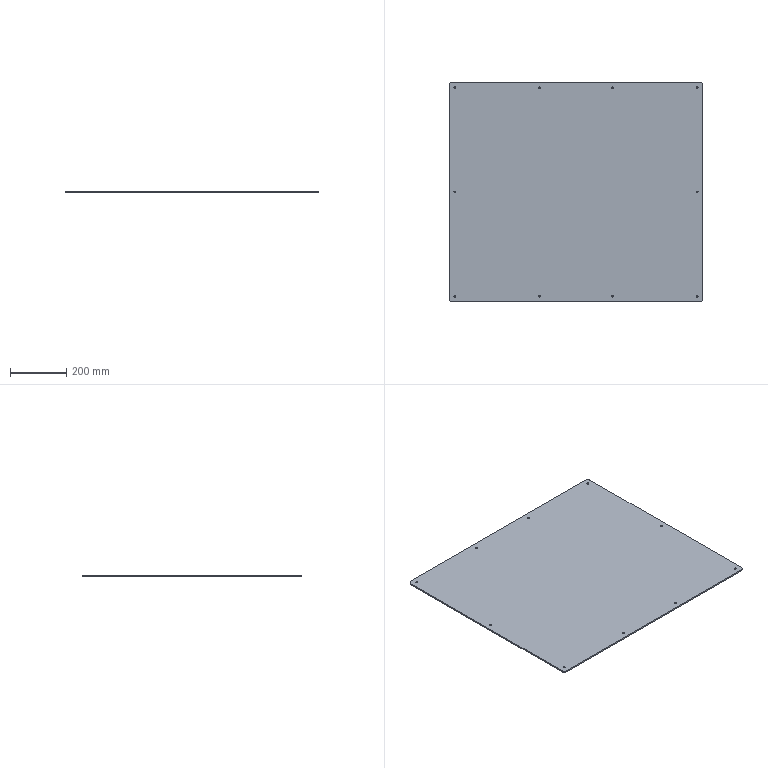Part | SolidWorks | features Extrusion 1, Fillet 1, HoleWzd 1 | 1 solid | 30 faces | box 900 x 780 x 5 mm | volume 3507647 mm3 | cylinder 24 | plane 6 | commonest cylinder face diameters 7 x20 20 x4
STEP:
#1=CARTESIAN_POINT('',(-426.5,370.,0.));
#2=VERTEX_POINT('',#1);
#3=CARTESIAN_POINT('',(-433.5,370.,0.));
#4=VERTEX_POINT('',#3);
#5=CARTESIAN_POINT('',(-430.,370.,0.));
#6=DIRECTION('',(0.,0.,-1.));
#7=DIRECTION('',(-1.,0.,0.));
#8=AXIS2_PLACEMENT_3D('',#5,#6,#7);
#9=CIRCLE('',#8,3.5);
#10=EDGE_CURVE('',#2,#4,#9,.T.);
#11=ORIENTED_EDGE('',*,*,#10,.T.);
#12=CARTESIAN_POINT('',(-433.5,370.,5.));
#13=VERTEX_POINT('',#12);
#14=CARTESIAN_POINT('',(-433.5,370.,5.));
#15=DIRECTION('',(0.,0.,1.));
#16=VECTOR('',#15,1000.);
#17=LINE('',#14,#16);
#18=EDGE_CURVE('',#4,#13,#17,.T.);
#19=ORIENTED_EDGE('',*,*,#18,.T.);
#20=CARTESIAN_POINT('',(-426.5,370.,5.));
#21=VERTEX_POINT('',#20);
#22=CARTESIAN_POINT('',(-430.,370.,5.));
#23=DIRECTION('',(0.,0.,1.));
#24=DIRECTION('',(1.,0.,0.));
#25=AXIS2_PLACEMENT_3D('',#22,#23,#24);
#26=CIRCLE('',#25,3.5);
#27=EDGE_CURVE('',#13,#21,#26,.T.);
#28=ORIENTED_EDGE('',*,*,#27,.T.);
#29=CARTESIAN_POINT('',(-426.5,370.,5.));
#30=DIRECTION('',(0.,0.,1.));
#31=VECTOR('',#30,1000.);
#32=LINE('',#29,#31);
#33=EDGE_CURVE('',#2,#21,#32,.T.);
#34=ORIENTED_EDGE('',*,*,#33,.F.);
#35=EDGE_LOOP('',(#11,#19,#28,#34));
#36=FACE_OUTER_BOUND('',#35,.T.);
#37=CARTESIAN_POINT('',(-430.,370.,5.));
#38=DIRECTION('',(0.,0.,1.));
#39=DIRECTION('',(1.,0.,0.));
#40=AXIS2_PLACEMENT_3D('',#37,#38,#39);
#41=CYLINDRICAL_SURFACE('',#40,3.5);
#42=ADVANCED_FACE('',(#36),#41,.F.);
#43=CARTESIAN_POINT('',(433.5,370.,0.));
#44=VERTEX_POINT('',#43);
#45=CARTESIAN_POINT('',(426.5,370.,0.));
#46=VERTEX_POINT('',#45);
#47=CARTESIAN_POINT('',(430.,370.,0.));
#48=DIRECTION('',(0.,0.,-1.));
#49=DIRECTION('',(-1.,0.,0.));
#50=AXIS2_PLACEMENT_3D('',#47,#48,#49);
#51=CIRCLE('',#50,3.5);
#52=EDGE_CURVE('',#44,#46,#51,.T.);
#53=ORIENTED_EDGE('',*,*,#52,.T.);
#54=CARTESIAN_POINT('',(426.5,370.,5.));
#55=VERTEX_POINT('',#54);
#56=CARTESIAN_POINT('',(426.5,370.,5.));
#57=DIRECTION('',(0.,0.,1.));
#58=VECTOR('',#57,1000.);
#59=LINE('',#56,#58);
#60=EDGE_CURVE('',#46,#55,#59,.T.);
#61=ORIENTED_EDGE('',*,*,#60,.T.);
#62=CARTESIAN_POINT('',(433.5,370.,5.));
#63=VERTEX_POINT('',#62);
#64=CARTESIAN_POINT('',(430.,370.,5.));
#65=DIRECTION('',(0.,0.,1.));
#66=DIRECTION('',(1.,0.,0.));
#67=AXIS2_PLACEMENT_3D('',#64,#65,#66);
#68=CIRCLE('',#67,3.5);
#69=EDGE_CURVE('',#55,#63,#68,.T.);
#70=ORIENTED_EDGE('',*,*,#69,.T.);
#71=CARTESIAN_POINT('',(433.5,370.,5.));
#72=DIRECTION('',(0.,0.,1.));
#73=VECTOR('',#72,1000.);
#74=LINE('',#71,#73);
#75=EDGE_CURVE('',#44,#63,#74,.T.);
#76=ORIENTED_EDGE('',*,*,#75,.F.);
#77=EDGE_LOOP('',(#53,#61,#70,#76));
#78=FACE_OUTER_BOUND('',#77,.T.);
#79=CARTESIAN_POINT('',(430.,370.,5.));
#80=DIRECTION('',(0.,0.,1.));
#81=DIRECTION('',(1.,0.,0.));
#82=AXIS2_PLACEMENT_3D('',#79,#80,#81);
#83=CYLINDRICAL_SURFACE('',#82,3.5);
#84=ADVANCED_FACE('',(#78),#83,.F.);
#85=CARTESIAN_POINT('',(433.5,-370.,0.));
#86=VERTEX_POINT('',#85);
#87=CARTESIAN_POINT('',(426.5,-370.,0.));
#88=VERTEX_POINT('',#87);
#89=CARTESIAN_POINT('',(430.,-370.,0.));
#90=DIRECTION('',(0.,0.,-1.));
#91=DIRECTION('',(-1.,0.,0.));
#92=AXIS2_PLACEMENT_3D('',#89,#90,#91);
#93=CIRCLE('',#92,3.5);
#94=EDGE_CURVE('',#86,#88,#93,.T.);
#95=ORIENTED_EDGE('',*,*,#94,.T.);
#96=CARTESIAN_POINT('',(426.5,-370.,5.));
#97=VERTEX_POINT('',#96);
#98=CARTESIAN_POINT('',(426.5,-370.,5.));
#99=DIRECTION('',(0.,0.,1.));
#100=VECTOR('',#99,1000.);
#101=LINE('',#98,#100);
#102=EDGE_CURVE('',#88,#97,#101,.T.);
#103=ORIENTED_EDGE('',*,*,#102,.T.);
#104=CARTESIAN_POINT('',(433.5,-370.,5.));
#105=VERTEX_POINT('',#104);
#106=CARTESIAN_POINT('',(430.,-370.,5.));
#107=DIRECTION('',(0.,0.,1.));
#108=DIRECTION('',(1.,0.,0.));
#109=AXIS2_PLACEMENT_3D('',#106,#107,#108);
#110=CIRCLE('',#109,3.5);
#111=EDGE_CURVE('',#97,#105,#110,.T.);
#112=ORIENTED_EDGE('',*,*,#111,.T.);
#113=CARTESIAN_POINT('',(433.5,-370.,5.));
#114=DIRECTION('',(0.,0.,1.));
#115=VECTOR('',#114,1000.);
#116=LINE('',#113,#115);
#117=EDGE_CURVE('',#86,#105,#116,.T.);
#118=ORIENTED_EDGE('',*,*,#117,.F.);
#119=EDGE_LOOP('',(#95,#103,#112,#118));
#120=FACE_OUTER_BOUND('',#119,.T.);
#121=CARTESIAN_POINT('',(430.,-370.,5.));
#122=DIRECTION('',(0.,0.,1.));
#123=DIRECTION('',(1.,0.,0.));
#124=AXIS2_PLACEMENT_3D('',#121,#122,#123);
#125=CYLINDRICAL_SURFACE('',#124,3.5);
#126=ADVANCED_FACE('',(#120),#125,.F.);
#127=CARTESIAN_POINT('',(-426.5,-370.,0.));
#128=VERTEX_POINT('',#127);
#129=CARTESIAN_POINT('',(-433.5,-370.,0.));
#130=VERTEX_POINT('',#129);
#131=CARTESIAN_POINT('',(-430.,-370.,0.));
#132=DIRECTION('',(0.,0.,-1.));
#133=DIRECTION('',(-1.,0.,0.));
#134=AXIS2_PLACEMENT_3D('',#131,#132,#133);
#135=CIRCLE('',#134,3.5);
#136=EDGE_CURVE('',#128,#130,#135,.T.);
#137=ORIENTED_EDGE('',*,*,#136,.T.);
#138=CARTESIAN_POINT('',(-433.5,-370.,5.));
#139=VERTEX_POINT('',#138);
#140=CARTESIAN_POINT('',(-433.5,-370.,5.));
#141=DIRECTION('',(0.,0.,1.));
#142=VECTOR('',#141,1000.);
#143=LINE('',#140,#142);
#144=EDGE_CURVE('',#130,#139,#143,.T.);
#145=ORIENTED_EDGE('',*,*,#144,.T.);
#146=CARTESIAN_POINT('',(-426.5,-370.,5.));
#147=VERTEX_POINT('',#146);
#148=CARTESIAN_POINT('',(-430.,-370.,5.));
#149=DIRECTION('',(0.,0.,1.));
#150=DIRECTION('',(1.,0.,0.));
#151=AXIS2_PLACEMENT_3D('',#148,#149,#150);
#152=CIRCLE('',#151,3.5);
#153=EDGE_CURVE('',#139,#147,#152,.T.);
#154=ORIENTED_EDGE('',*,*,#153,.T.);
#155=CARTESIAN_POINT('',(-426.5,-370.,5.));
#156=DIRECTION('',(0.,0.,1.));
#157=VECTOR('',#156,1000.);
#158=LINE('',#155,#157);
#159=EDGE_CURVE('',#128,#147,#158,.T.);
#160=ORIENTED_EDGE('',*,*,#159,.F.);
#161=EDGE_LOOP('',(#137,#145,#154,#160));
#162=FACE_OUTER_BOUND('',#161,.T.);
#163=CARTESIAN_POINT('',(-430.,-370.,5.));
#164=DIRECTION('',(0.,0.,1.));
#165=DIRECTION('',(1.,0.,0.));
#166=AXIS2_PLACEMENT_3D('',#163,#164,#165);
#167=CYLINDRICAL_SURFACE('',#166,3.5);
#168=ADVANCED_FACE('',(#162),#167,.F.);
#169=CARTESIAN_POINT('',(-426.5,0.,0.));
#170=VERTEX_POINT('',#169);
#171=CARTESIAN_POINT('',(-433.5,0.,0.));
#172=VERTEX_POINT('',#171);
#173=CARTESIAN_POINT('',(-430.,0.,0.));
#174=DIRECTION('',(0.,0.,-1.));
#175=DIRECTION('',(-1.,0.,0.));
#176=AXIS2_PLACEMENT_3D('',#173,#174,#175);
#177=CIRCLE('',#176,3.5);
#178=EDGE_CURVE('',#170,#172,#177,.T.);
#179=ORIENTED_EDGE('',*,*,#178,.T.);
#180=CARTESIAN_POINT('',(-433.5,0.,5.));
#181=VERTEX_POINT('',#180);
#182=CARTESIAN_POINT('',(-433.5,0.,5.));
#183=DIRECTION('',(0.,0.,1.));
#184=VECTOR('',#183,1000.);
#185=LINE('',#182,#184);
#186=EDGE_CURVE('',#172,#181,#185,.T.);
#187=ORIENTED_EDGE('',*,*,#186,.T.);
#188=CARTESIAN_POINT('',(-426.5,0.,5.));
#189=VERTEX_POINT('',#188);
#190=CARTESIAN_POINT('',(-430.,0.,5.));
#191=DIRECTION('',(0.,0.,1.));
#192=DIRECTION('',(1.,0.,0.));
#193=AXIS2_PLACEMENT_3D('',#190,#191,#192);
#194=CIRCLE('',#193,3.5);
#195=EDGE_CURVE('',#181,#189,#194,.T.);
#196=ORIENTED_EDGE('',*,*,#195,.T.);
#197=CARTESIAN_POINT('',(-426.5,0.,5.));
#198=DIRECTION('',(0.,0.,1.));
#199=VECTOR('',#198,1000.);
#200=LINE('',#197,#199);
#201=EDGE_CURVE('',#170,#189,#200,.T.);
#202=ORIENTED_EDGE('',*,*,#201,.F.);
#203=EDGE_LOOP('',(#179,#187,#196,#202));
#204=FACE_OUTER_BOUND('',#203,.T.);
#205=CARTESIAN_POINT('',(-430.,0.,5.));
#206=DIRECTION('',(0.,0.,1.));
#207=DIRECTION('',(1.,0.,0.));
#208=AXIS2_PLACEMENT_3D('',#205,#206,#207);
#209=CYLINDRICAL_SURFACE('',#208,3.5);
#210=ADVANCED_FACE('',(#204),#209,.F.);
#211=CARTESIAN_POINT('',(433.5,0.,0.));
#212=VERTEX_POINT('',#211);
#213=CARTESIAN_POINT('',(426.5,0.,0.));
#214=VERTEX_POINT('',#213);
#215=CARTESIAN_POINT('',(430.,0.,0.));
#216=DIRECTION('',(0.,0.,-1.));
#217=DIRECTION('',(-1.,0.,0.));
#218=AXIS2_PLACEMENT_3D('',#215,#216,#217);
#219=CIRCLE('',#218,3.5);
#220=EDGE_CURVE('',#212,#214,#219,.T.);
#221=ORIENTED_EDGE('',*,*,#220,.T.);
#222=CARTESIAN_POINT('',(426.5,0.,5.));
#223=VERTEX_POINT('',#222);
#224=CARTESIAN_POINT('',(426.5,0.,5.));
#225=DIRECTION('',(0.,0.,1.));
#226=VECTOR('',#225,1000.);
#227=LINE('',#224,#226);
#228=EDGE_CURVE('',#214,#223,#227,.T.);
#229=ORIENTED_EDGE('',*,*,#228,.T.);
#230=CARTESIAN_POINT('',(433.5,0.,5.));
#231=VERTEX_POINT('',#230);
#232=CARTESIAN_POINT('',(430.,0.,5.));
#233=DIRECTION('',(0.,0.,1.));
#234=DIRECTION('',(1.,0.,0.));
#235=AXIS2_PLACEMENT_3D('',#232,#233,#234);
#236=CIRCLE('',#235,3.5);
#237=EDGE_CURVE('',#223,#231,#236,.T.);
#238=ORIENTED_EDGE('',*,*,#237,.T.);
#239=CARTESIAN_POINT('',(433.5,0.,5.));
#240=DIRECTION('',(0.,0.,1.));
#241=VECTOR('',#240,1000.);
#242=LINE('',#239,#241);
#243=EDGE_CURVE('',#212,#231,#242,.T.);
#244=ORIENTED_EDGE('',*,*,#243,.F.);
#245=EDGE_LOOP('',(#221,#229,#238,#244));
#246=FACE_OUTER_BOUND('',#245,.T.);
#247=CARTESIAN_POINT('',(430.,0.,5.));
#248=DIRECTION('',(0.,0.,1.));
#249=DIRECTION('',(1.,0.,0.));
#250=AXIS2_PLACEMENT_3D('',#247,#248,#249);
#251=CYLINDRICAL_SURFACE('',#250,3.5);
#252=ADVANCED_FACE('',(#246),#251,.F.);
#253=CARTESIAN_POINT('',(-126.5,370.,0.));
#254=VERTEX_POINT('',#253);
#255=CARTESIAN_POINT('',(-133.5,370.,0.));
#256=VERTEX_POINT('',#255);
#257=CARTESIAN_POINT('',(-130.,370.,0.));
#258=DIRECTION('',(0.,0.,-1.));
#259=DIRECTION('',(-1.,0.,0.));
#260=AXIS2_PLACEMENT_3D('',#257,#258,#259);
#261=CIRCLE('',#260,3.5);
#262=EDGE_CURVE('',#254,#256,#261,.T.);
#263=ORIENTED_EDGE('',*,*,#262,.T.);
#264=CARTESIAN_POINT('',(-133.5,370.,5.));
#265=VERTEX_POINT('',#264);
#266=CARTESIAN_POINT('',(-133.5,370.,5.));
#267=DIRECTION('',(0.,0.,1.));
#268=VECTOR('',#267,1000.);
#269=LINE('',#266,#268);
#270=EDGE_CURVE('',#256,#265,#269,.T.);
#271=ORIENTED_EDGE('',*,*,#270,.T.);
#272=CARTESIAN_POINT('',(-126.5,370.,5.));
#273=VERTEX_POINT('',#272);
#274=CARTESIAN_POINT('',(-130.,370.,5.));
#275=DIRECTION('',(0.,0.,1.));
#276=DIRECTION('',(1.,0.,0.));
#277=AXIS2_PLACEMENT_3D('',#274,#275,#276);
#278=CIRCLE('',#277,3.5);
#279=EDGE_CURVE('',#265,#273,#278,.T.);
#280=ORIENTED_EDGE('',*,*,#279,.T.);
#281=CARTESIAN_POINT('',(-126.5,370.,5.));
#282=DIRECTION('',(0.,0.,1.));
#283=VECTOR('',#282,1000.);
#284=LINE('',#281,#283);
#285=EDGE_CURVE('',#254,#273,#284,.T.);
#286=ORIENTED_EDGE('',*,*,#285,.F.);
#287=EDGE_LOOP('',(#263,#271,#280,#286));
#288=FACE_OUTER_BOUND('',#287,.T.);
#289=CARTESIAN_POINT('',(-130.,370.,5.));
#290=DIRECTION('',(0.,0.,1.));
#291=DIRECTION('',(1.,0.,0.));
#292=AXIS2_PLACEMENT_3D('',#289,#290,#291);
#293=CYLINDRICAL_SURFACE('',#292,3.5);
#294=ADVANCED_FACE('',(#288),#293,.F.);
#295=CARTESIAN_POINT('',(133.5,370.,0.));
#296=VERTEX_POINT('',#295);
#297=CARTESIAN_POINT('',(126.5,370.,0.));
#298=VERTEX_POINT('',#297);
#299=CARTESIAN_POINT('',(130.,370.,0.));
#300=DIRECTION('',(0.,0.,-1.));
#301=DIRECTION('',(-1.,0.,0.));
#302=AXIS2_PLACEMENT_3D('',#299,#300,#301);
#303=CIRCLE('',#302,3.5);
#304=EDGE_CURVE('',#296,#298,#303,.T.);
#305=ORIENTED_EDGE('',*,*,#304,.T.);
#306=CARTESIAN_POINT('',(126.5,370.,5.));
#307=VERTEX_POINT('',#306);
#308=CARTESIAN_POINT('',(126.5,370.,5.));
#309=DIRECTION('',(0.,0.,1.));
#310=VECTOR('',#309,1000.);
#311=LINE('',#308,#310);
#312=EDGE_CURVE('',#298,#307,#311,.T.);
#313=ORIENTED_EDGE('',*,*,#312,.T.);
#314=CARTESIAN_POINT('',(133.5,370.,5.));
#315=VERTEX_POINT('',#314);
#316=CARTESIAN_POINT('',(130.,370.,5.));
#317=DIRECTION('',(0.,0.,1.));
#318=DIRECTION('',(1.,0.,0.));
#319=AXIS2_PLACEMENT_3D('',#316,#317,#318);
#320=CIRCLE('',#319,3.5);
#321=EDGE_CURVE('',#307,#315,#320,.T.);
#322=ORIENTED_EDGE('',*,*,#321,.T.);
#323=CARTESIAN_POINT('',(133.5,370.,5.));
#324=DIRECTION('',(0.,0.,1.));
#325=VECTOR('',#324,1000.);
#326=LINE('',#323,#325);
#327=EDGE_CURVE('',#296,#315,#326,.T.);
#328=ORIENTED_EDGE('',*,*,#327,.F.);
#329=EDGE_LOOP('',(#305,#313,#322,#328));
#330=FACE_OUTER_BOUND('',#329,.T.);
#331=CARTESIAN_POINT('',(130.,370.,5.));
#332=DIRECTION('',(0.,0.,1.));
#333=DIRECTION('',(1.,0.,0.));
#334=AXIS2_PLACEMENT_3D('',#331,#332,#333);
#335=CYLINDRICAL_SURFACE('',#334,3.5);
#336=ADVANCED_FACE('',(#330),#335,.F.);
#337=CARTESIAN_POINT('',(-126.5,-370.,0.));
#338=VERTEX_POINT('',#337);
#339=CARTESIAN_POINT('',(-133.5,-370.,0.));
#340=VERTEX_POINT('',#339);
#341=CARTESIAN_POINT('',(-130.,-370.,0.));
#342=DIRECTION('',(0.,0.,-1.));
#343=DIRECTION('',(-1.,0.,0.));
#344=AXIS2_PLACEMENT_3D('',#341,#342,#343);
#345=CIRCLE('',#344,3.5);
#346=EDGE_CURVE('',#338,#340,#345,.T.);
#347=ORIENTED_EDGE('',*,*,#346,.T.);
#348=CARTESIAN_POINT('',(-133.5,-370.,5.));
#349=VERTEX_POINT('',#348);
#350=CARTESIAN_POINT('',(-133.5,-370.,5.));
#351=DIRECTION('',(0.,0.,1.));
#352=VECTOR('',#351,1000.);
#353=LINE('',#350,#352);
#354=EDGE_CURVE('',#340,#349,#353,.T.);
#355=ORIENTED_EDGE('',*,*,#354,.T.);
#356=CARTESIAN_POINT('',(-126.5,-370.,5.));
#357=VERTEX_POINT('',#356);
#358=CARTESIAN_POINT('',(-130.,-370.,5.));
#359=DIRECTION('',(0.,0.,1.));
#360=DIRECTION('',(1.,0.,0.));
#361=AXIS2_PLACEMENT_3D('',#358,#359,#360);
#362=CIRCLE('',#361,3.5);
#363=EDGE_CURVE('',#349,#357,#362,.T.);
#364=ORIENTED_EDGE('',*,*,#363,.T.);
#365=CARTESIAN_POINT('',(-126.5,-370.,5.));
#366=DIRECTION('',(0.,0.,1.));
#367=VECTOR('',#366,1000.);
#368=LINE('',#365,#367);
#369=EDGE_CURVE('',#338,#357,#368,.T.);
#370=ORIENTED_EDGE('',*,*,#369,.F.);
#371=EDGE_LOOP('',(#347,#355,#364,#370));
#372=FACE_OUTER_BOUND('',#371,.T.);
#373=CARTESIAN_POINT('',(-130.,-370.,5.));
#374=DIRECTION('',(0.,0.,1.));
#375=DIRECTION('',(1.,0.,0.));
#376=AXIS2_PLACEMENT_3D('',#373,#374,#375);
#377=CYLINDRICAL_SURFACE('',#376,3.5);
#378=ADVANCED_FACE('',(#372),#377,.F.);
#379=CARTESIAN_POINT('',(133.5,-370.,0.));
#380=VERTEX_POINT('',#379);
#381=CARTESIAN_POINT('',(126.5,-370.,0.));
#382=VERTEX_POINT('',#381);
#383=CARTESIAN_POINT('',(130.,-370.,0.));
#384=DIRECTION('',(0.,0.,-1.));
#385=DIRECTION('',(-1.,0.,0.));
#386=AXIS2_PLACEMENT_3D('',#383,#384,#385);
#387=CIRCLE('',#386,3.5);
#388=EDGE_CURVE('',#380,#382,#387,.T.);
#389=ORIENTED_EDGE('',*,*,#388,.T.);
#390=CARTESIAN_POINT('',(126.5,-370.,5.));
#391=VERTEX_POINT('',#390);
#392=CARTESIAN_POINT('',(126.5,-370.,5.));
#393=DIRECTION('',(0.,0.,1.));
#394=VECTOR('',#393,1000.);
#395=LINE('',#392,#394);
#396=EDGE_CURVE('',#382,#391,#395,.T.);
#397=ORIENTED_EDGE('',*,*,#396,.T.);
#398=CARTESIAN_POINT('',(133.5,-370.,5.));
#399=VERTEX_POINT('',#398);
#400=CARTESIAN_POINT('',(130.,-370.,5.));
#401=DIRECTION('',(0.,0.,1.));
#402=DIRECTION('',(1.,0.,0.));
#403=AXIS2_PLACEMENT_3D('',#400,#401,#402);
#404=CIRCLE('',#403,3.5);
#405=EDGE_CURVE('',#391,#399,#404,.T.);
#406=ORIENTED_EDGE('',*,*,#405,.T.);
#407=CARTESIAN_POINT('',(133.5,-370.,5.));
#408=DIRECTION('',(0.,0.,1.));
#409=VECTOR('',#408,1000.);
#410=LINE('',#407,#409);
#411=EDGE_CURVE('',#380,#399,#410,.T.);
#412=ORIENTED_EDGE('',*,*,#411,.F.);
#413=EDGE_LOOP('',(#389,#397,#406,#412));
#414=FACE_OUTER_BOUND('',#413,.T.);
#415=CARTESIAN_POINT('',(130.,-370.,5.));
#416=DIRECTION('',(0.,0.,1.));
#417=DIRECTION('',(1.,0.,0.));
#418=AXIS2_PLACEMENT_3D('',#415,#416,#417);
#419=CYLINDRICAL_SURFACE('',#418,3.5);
#420=ADVANCED_FACE('',(#414),#419,.F.);
#421=CARTESIAN_POINT('',(450.,-380.,5.));
#422=VERTEX_POINT('',#421);
#423=CARTESIAN_POINT('',(450.,380.,5.));
#424=VERTEX_POINT('',#423);
#425=CARTESIAN_POINT('',(450.,-390.,5.));
#426=DIRECTION('',(0.,1.,0.));
#427=VECTOR('',#426,1000.);
#428=LINE('',#425,#427);
#429=EDGE_CURVE('',#422,#424,#428,.T.);
#430=ORIENTED_EDGE('',*,*,#429,.F.);
#431=CARTESIAN_POINT('',(450.,-380.,0.));
#432=VERTEX_POINT('',#431);
#433=CARTESIAN_POINT('',(450.,-380.,5.));
#434=DIRECTION('',(0.,0.,-1.));
#435=VECTOR('',#434,1000.);
#436=LINE('',#433,#435);
#437=EDGE_CURVE('',#422,#432,#436,.T.);
#438=ORIENTED_EDGE('',*,*,#437,.T.);
#439=CARTESIAN_POINT('',(450.,380.,0.));
#440=VERTEX_POINT('',#439);
#441=CARTESIAN_POINT('',(450.,-390.,0.));
#442=DIRECTION('',(0.,1.,0.));
#443=VECTOR('',#442,1000.);
#444=LINE('',#441,#443);
#445=EDGE_CURVE('',#432,#440,#444,.T.);
#446=ORIENTED_EDGE('',*,*,#445,.T.);
#447=CARTESIAN_POINT('',(450.,380.,5.));
#448=DIRECTION('',(0.,0.,1.));
#449=VECTOR('',#448,1000.);
#450=LINE('',#447,#449);
#451=EDGE_CURVE('',#440,#424,#450,.T.);
#452=ORIENTED_EDGE('',*,*,#451,.T.);
#453=EDGE_LOOP('',(#430,#438,#446,#452));
#454=FACE_OUTER_BOUND('',#453,.T.);
#455=CARTESIAN_POINT('',(450.,-390.,5.));
#456=DIRECTION('',(-1.,0.,0.));
#457=DIRECTION('',(0.,0.,1.));
#458=AXIS2_PLACEMENT_3D('',#455,#456,#457);
#459=PLANE('',#458);
#460=ADVANCED_FACE('',(#454),#459,.F.);
#461=CARTESIAN_POINT('',(440.,390.,5.));
#462=VERTEX_POINT('',#461);
#463=CARTESIAN_POINT('',(-440.,390.,5.));
#464=VERTEX_POINT('',#463);
#465=CARTESIAN_POINT('',(-450.,390.,5.));
#466=DIRECTION('',(-1.,0.,0.));
#467=VECTOR('',#466,1000.);
#468=LINE('',#465,#467);
#469=EDGE_CURVE('',#462,#464,#468,.T.);
#470=ORIENTED_EDGE('',*,*,#469,.F.);
#471=CARTESIAN_POINT('',(440.,390.,0.));
#472=VERTEX_POINT('',#471);
#473=CARTESIAN_POINT('',(440.,390.,5.));
#474=DIRECTION('',(0.,0.,-1.));
#475=VECTOR('',#474,1000.);
#476=LINE('',#473,#475);
#477=EDGE_CURVE('',#462,#472,#476,.T.);
#478=ORIENTED_EDGE('',*,*,#477,.T.);
#479=CARTESIAN_POINT('',(-440.,390.,0.));
#480=VERTEX_POINT('',#479);
#481=CARTESIAN_POINT('',(-450.,390.,0.));
#482=DIRECTION('',(-1.,0.,0.));
#483=VECTOR('',#482,1000.);
#484=LINE('',#481,#483);
#485=EDGE_CURVE('',#472,#480,#484,.T.);
#486=ORIENTED_EDGE('',*,*,#485,.T.);
#487=CARTESIAN_POINT('',(-440.,390.,5.));
#488=DIRECTION('',(0.,0.,1.));
#489=VECTOR('',#488,1000.);
#490=LINE('',#487,#489);
#491=EDGE_CURVE('',#480,#464,#490,.T.);
#492=ORIENTED_EDGE('',*,*,#491,.T.);
#493=EDGE_LOOP('',(#470,#478,#486,#492));
#494=FACE_OUTER_BOUND('',#493,.T.);
#495=CARTESIAN_POINT('',(-450.,390.,5.));
#496=DIRECTION('',(0.,-1.,0.));
#497=DIRECTION('',(0.,0.,-1.));
#498=AXIS2_PLACEMENT_3D('',#495,#496,#497);
#499=PLANE('',#498);
#500=ADVANCED_FACE('',(#494),#499,.F.);
#501=CARTESIAN_POINT('',(-450.,380.,0.));
#502=VERTEX_POINT('',#501);
#503=CARTESIAN_POINT('',(-450.,-380.,0.));
#504=VERTEX_POINT('',#503);
#505=CARTESIAN_POINT('',(-450.,-390.,0.));
#506=DIRECTION('',(0.,-1.,0.));
#507=VECTOR('',#506,1000.);
#508=LINE('',#505,#507);
#509=EDGE_CURVE('',#502,#504,#508,.T.);
#510=ORIENTED_EDGE('',*,*,#509,.T.);
#511=CARTESIAN_POINT('',(-450.,-380.,5.));
#512=VERTEX_POINT('',#511);
#513=CARTESIAN_POINT('',(-450.,-380.,5.));
#514=DIRECTION('',(0.,0.,1.));
#515=VECTOR('',#514,1000.);
#516=LINE('',#513,#515);
#517=EDGE_CURVE('',#504,#512,#516,.T.);
#518=ORIENTED_EDGE('',*,*,#517,.T.);
#519=CARTESIAN_POINT('',(-450.,380.,5.));
#520=VERTEX_POINT('',#519);
#521=CARTESIAN_POINT('',(-450.,-390.,5.));
#522=DIRECTION('',(0.,-1.,0.));
#523=VECTOR('',#522,1000.);
#524=LINE('',#521,#523);
#525=EDGE_CURVE('',#520,#512,#524,.T.);
#526=ORIENTED_EDGE('',*,*,#525,.F.);
#527=CARTESIAN_POINT('',(-450.,380.,5.));
#528=DIRECTION('',(0.,0.,-1.));
#529=VECTOR('',#528,1000.);
#530=LINE('',#527,#529);
#531=EDGE_CURVE('',#520,#502,#530,.T.);
#532=ORIENTED_EDGE('',*,*,#531,.T.);
#533=EDGE_LOOP('',(#510,#518,#526,#532));
#534=FACE_OUTER_BOUND('',#533,.T.);
#535=CARTESIAN_POINT('',(-450.,-390.,5.));
#536=DIRECTION('',(1.,0.,0.));
#537=DIRECTION('',(0.,0.,-1.));
#538=AXIS2_PLACEMENT_3D('',#535,#536,#537);
#539=PLANE('',#538);
#540=ADVANCED_FACE('',(#534),#539,.F.);
#541=CARTESIAN_POINT('',(-440.,-390.,5.));
#542=VERTEX_POINT('',#541);
#543=CARTESIAN_POINT('',(440.,-390.,5.));
#544=VERTEX_POINT('',#543);
#545=CARTESIAN_POINT('',(-450.,-390.,5.));
#546=DIRECTION('',(1.,0.,0.));
#547=VECTOR('',#546,1000.);
#548=LINE('',#545,#547);
#549=EDGE_CURVE('',#542,#544,#548,.T.);
#550=ORIENTED_EDGE('',*,*,#549,.F.);
#551=CARTESIAN_POINT('',(-440.,-390.,0.));
#552=VERTEX_POINT('',#551);
#553=CARTESIAN_POINT('',(-440.,-390.,5.));
#554=DIRECTION('',(0.,0.,-1.));
#555=VECTOR('',#554,1000.);
#556=LINE('',#553,#555);
#557=EDGE_CURVE('',#542,#552,#556,.T.);
#558=ORIENTED_EDGE('',*,*,#557,.T.);
#559=CARTESIAN_POINT('',(440.,-390.,0.));
#560=VERTEX_POINT('',#559);
#561=CARTESIAN_POINT('',(-450.,-390.,0.));
#562=DIRECTION('',(1.,0.,0.));
#563=VECTOR('',#562,1000.);
#564=LINE('',#561,#563);
#565=EDGE_CURVE('',#552,#560,#564,.T.);
#566=ORIENTED_EDGE('',*,*,#565,.T.);
#567=CARTESIAN_POINT('',(440.,-390.,5.));
#568=DIRECTION('',(0.,0.,1.));
#569=VECTOR('',#568,1000.);
#570=LINE('',#567,#569);
#571=EDGE_CURVE('',#560,#544,#570,.T.);
#572=ORIENTED_EDGE('',*,*,#571,.T.);
#573=EDGE_LOOP('',(#550,#558,#566,#572));
#574=FACE_OUTER_BOUND('',#573,.T.);
#575=CARTESIAN_POINT('',(-450.,-390.,5.));
#576=DIRECTION('',(0.,1.,0.));
#577=DIRECTION('',(0.,0.,1.));
#578=AXIS2_PLACEMENT_3D('',#575,#576,#577);
#579=PLANE('',#578);
#580=ADVANCED_FACE('',(#574),#579,.F.);
#581=CARTESIAN_POINT('',(-430.,370.,5.));
#582=DIRECTION('',(0.,0.,1.));
#583=DIRECTION('',(1.,0.,0.));
#584=AXIS2_PLACEMENT_3D('',#581,#582,#583);
#585=CIRCLE('',#584,3.5);
#586=EDGE_CURVE('',#21,#13,#585,.T.);
#587=ORIENTED_EDGE('',*,*,#586,.F.);
#588=ORIENTED_EDGE('',*,*,#27,.F.);
#589=EDGE_LOOP('',(#587,#588));
#590=FACE_BOUND('',#589,.T.);
#591=CARTESIAN_POINT('',(430.,370.,5.));
#592=DIRECTION('',(0.,0.,1.));
#593=DIRECTION('',(1.,0.,0.));
#594=AXIS2_PLACEMENT_3D('',#591,#592,#593);
#595=CIRCLE('',#594,3.5);
#596=EDGE_CURVE('',#63,#55,#595,.T.);
#597=ORIENTED_EDGE('',*,*,#596,.F.);
#598=ORIENTED_EDGE('',*,*,#69,.F.);
#599=EDGE_LOOP('',(#597,#598));
#600=FACE_BOUND('',#599,.T.);
#601=CARTESIAN_POINT('',(430.,-370.,5.));
#602=DIRECTION('',(0.,0.,1.));
#603=DIRECTION('',(1.,0.,0.));
#604=AXIS2_PLACEMENT_3D('',#601,#602,#603);
#605=CIRCLE('',#604,3.5);
#606=EDGE_CURVE('',#105,#97,#605,.T.);
#607=ORIENTED_EDGE('',*,*,#606,.F.);
#608=ORIENTED_EDGE('',*,*,#111,.F.);
#609=EDGE_LOOP('',(#607,#608));
#610=FACE_BOUND('',#609,.T.);
#611=CARTESIAN_POINT('',(-430.,-370.,5.));
#612=DIRECTION('',(0.,0.,1.));
#613=DIRECTION('',(1.,0.,0.));
#614=AXIS2_PLACEMENT_3D('',#611,#612,#613);
#615=CIRCLE('',#614,3.5);
#616=EDGE_CURVE('',#147,#139,#615,.T.);
#617=ORIENTED_EDGE('',*,*,#616,.F.);
#618=ORIENTED_EDGE('',*,*,#153,.F.);
#619=EDGE_LOOP('',(#617,#618));
#620=FACE_BOUND('',#619,.T.);
#621=CARTESIAN_POINT('',(-430.,0.,5.));
#622=DIRECTION('',(0.,0.,1.));
#623=DIRECTION('',(1.,0.,0.));
#624=AXIS2_PLACEMENT_3D('',#621,#622,#623);
#625=CIRCLE('',#624,3.5);
#626=EDGE_CURVE('',#189,#181,#625,.T.);
#627=ORIENTED_EDGE('',*,*,#626,.F.);
#628=ORIENTED_EDGE('',*,*,#195,.F.);
#629=EDGE_LOOP('',(#627,#628));
#630=FACE_BOUND('',#629,.T.);
#631=CARTESIAN_POINT('',(430.,0.,5.));
#632=DIRECTION('',(0.,0.,1.));
#633=DIRECTION('',(1.,0.,0.));
#634=AXIS2_PLACEMENT_3D('',#631,#632,#633);
#635=CIRCLE('',#634,3.5);
#636=EDGE_CURVE('',#231,#223,#635,.T.);
#637=ORIENTED_EDGE('',*,*,#636,.F.);
#638=ORIENTED_EDGE('',*,*,#237,.F.);
#639=EDGE_LOOP('',(#637,#638));
#640=FACE_BOUND('',#639,.T.);
#641=CARTESIAN_POINT('',(-130.,370.,5.));
#642=DIRECTION('',(0.,0.,1.));
#643=DIRECTION('',(1.,0.,0.));
#644=AXIS2_PLACEMENT_3D('',#641,#642,#643);
#645=CIRCLE('',#644,3.5);
#646=EDGE_CURVE('',#273,#265,#645,.T.);
#647=ORIENTED_EDGE('',*,*,#646,.F.);
#648=ORIENTED_EDGE('',*,*,#279,.F.);
#649=EDGE_LOOP('',(#647,#648));
#650=FACE_BOUND('',#649,.T.);
#651=CARTESIAN_POINT('',(130.,370.,5.));
#652=DIRECTION('',(0.,0.,1.));
#653=DIRECTION('',(1.,0.,0.));
#654=AXIS2_PLACEMENT_3D('',#651,#652,#653);
#655=CIRCLE('',#654,3.5);
#656=EDGE_CURVE('',#315,#307,#655,.T.);
#657=ORIENTED_EDGE('',*,*,#656,.F.);
#658=ORIENTED_EDGE('',*,*,#321,.F.);
#659=EDGE_LOOP('',(#657,#658));
#660=FACE_BOUND('',#659,.T.);
#661=CARTESIAN_POINT('',(-130.,-370.,5.));
#662=DIRECTION('',(0.,0.,1.));
#663=DIRECTION('',(1.,0.,0.));
#664=AXIS2_PLACEMENT_3D('',#661,#662,#663);
#665=CIRCLE('',#664,3.5);
#666=EDGE_CURVE('',#357,#349,#665,.T.);
#667=ORIENTED_EDGE('',*,*,#666,.F.);
#668=ORIENTED_EDGE('',*,*,#363,.F.);
#669=EDGE_LOOP('',(#667,#668));
#670=FACE_BOUND('',#669,.T.);
#671=CARTESIAN_POINT('',(130.,-370.,5.));
#672=DIRECTION('',(0.,0.,1.));
#673=DIRECTION('',(1.,0.,0.));
#674=AXIS2_PLACEMENT_3D('',#671,#672,#673);
#675=CIRCLE('',#674,3.5);
#676=EDGE_CURVE('',#399,#391,#675,.T.);
#677=ORIENTED_EDGE('',*,*,#676,.F.);
#678=ORIENTED_EDGE('',*,*,#405,.F.);
#679=EDGE_LOOP('',(#677,#678));
#680=FACE_BOUND('',#679,.T.);
#681=ORIENTED_EDGE('',*,*,#525,.T.);
#682=CARTESIAN_POINT('',(-440.,-380.,5.));
#683=DIRECTION('',(0.,0.,1.));
#684=DIRECTION('',(-1.,0.,0.));
#685=AXIS2_PLACEMENT_3D('',#682,#683,#684);
#686=CIRCLE('',#685,10.);
#687=EDGE_CURVE('',#512,#542,#686,.T.);
#688=ORIENTED_EDGE('',*,*,#687,.T.);
#689=ORIENTED_EDGE('',*,*,#549,.T.);
#690=CARTESIAN_POINT('',(440.,-380.,5.));
#691=DIRECTION('',(0.,0.,1.));
#692=DIRECTION('',(-1.,0.,0.));
#693=AXIS2_PLACEMENT_3D('',#690,#691,#692);
#694=CIRCLE('',#693,10.);
#695=EDGE_CURVE('',#544,#422,#694,.T.);
#696=ORIENTED_EDGE('',*,*,#695,.T.);
#697=ORIENTED_EDGE('',*,*,#429,.T.);
#698=CARTESIAN_POINT('',(440.,380.,5.));
#699=DIRECTION('',(0.,0.,1.));
#700=DIRECTION('',(-1.,0.,0.));
#701=AXIS2_PLACEMENT_3D('',#698,#699,#700);
#702=CIRCLE('',#701,10.);
#703=EDGE_CURVE('',#424,#462,#702,.T.);
#704=ORIENTED_EDGE('',*,*,#703,.T.);
#705=ORIENTED_EDGE('',*,*,#469,.T.);
#706=CARTESIAN_POINT('',(-440.,380.,5.));
#707=DIRECTION('',(0.,0.,1.));
#708=DIRECTION('',(-1.,0.,0.));
#709=AXIS2_PLACEMENT_3D('',#706,#707,#708);
#710=CIRCLE('',#709,10.);
#711=EDGE_CURVE('',#464,#520,#710,.T.);
#712=ORIENTED_EDGE('',*,*,#711,.T.);
#713=EDGE_LOOP('',(#681,#688,#689,#696,#697,#704,#705,#712));
#714=FACE_OUTER_BOUND('',#713,.T.);
#715=CARTESIAN_POINT('',(0.,0.,5.));
#716=DIRECTION('',(0.,0.,-1.));
#717=DIRECTION('',(-1.,0.,0.));
#718=AXIS2_PLACEMENT_3D('',#715,#716,#717);
#719=PLANE('',#718);
#720=ADVANCED_FACE('',(#590,#600,#610,#620,#630,#640,#650,#660,#670,#680,#714),#719,.F.);
#721=ORIENTED_EDGE('',*,*,#10,.F.);
#722=CARTESIAN_POINT('',(-430.,370.,0.));
#723=DIRECTION('',(0.,0.,-1.));
#724=DIRECTION('',(-1.,0.,0.));
#725=AXIS2_PLACEMENT_3D('',#722,#723,#724);
#726=CIRCLE('',#725,3.5);
#727=EDGE_CURVE('',#4,#2,#726,.T.);
#728=ORIENTED_EDGE('',*,*,#727,.F.);
#729=EDGE_LOOP('',(#721,#728));
#730=FACE_BOUND('',#729,.T.);
#731=ORIENTED_EDGE('',*,*,#52,.F.);
#732=CARTESIAN_POINT('',(430.,370.,0.));
#733=DIRECTION('',(0.,0.,-1.));
#734=DIRECTION('',(-1.,0.,0.));
#735=AXIS2_PLACEMENT_3D('',#732,#733,#734);
#736=CIRCLE('',#735,3.5);
#737=EDGE_CURVE('',#46,#44,#736,.T.);
#738=ORIENTED_EDGE('',*,*,#737,.F.);
#739=EDGE_LOOP('',(#731,#738));
#740=FACE_BOUND('',#739,.T.);
#741=ORIENTED_EDGE('',*,*,#94,.F.);
#742=CARTESIAN_POINT('',(430.,-370.,0.));
#743=DIRECTION('',(0.,0.,-1.));
#744=DIRECTION('',(-1.,0.,0.));
#745=AXIS2_PLACEMENT_3D('',#742,#743,#744);
#746=CIRCLE('',#745,3.5);
#747=EDGE_CURVE('',#88,#86,#746,.T.);
#748=ORIENTED_EDGE('',*,*,#747,.F.);
#749=EDGE_LOOP('',(#741,#748));
#750=FACE_BOUND('',#749,.T.);
#751=ORIENTED_EDGE('',*,*,#136,.F.);
#752=CARTESIAN_POINT('',(-430.,-370.,0.));
#753=DIRECTION('',(0.,0.,-1.));
#754=DIRECTION('',(-1.,0.,0.));
#755=AXIS2_PLACEMENT_3D('',#752,#753,#754);
#756=CIRCLE('',#755,3.5);
#757=EDGE_CURVE('',#130,#128,#756,.T.);
#758=ORIENTED_EDGE('',*,*,#757,.F.);
#759=EDGE_LOOP('',(#751,#758));
#760=FACE_BOUND('',#759,.T.);
#761=ORIENTED_EDGE('',*,*,#178,.F.);
#762=CARTESIAN_POINT('',(-430.,0.,0.));
#763=DIRECTION('',(0.,0.,-1.));
#764=DIRECTION('',(-1.,0.,0.));
#765=AXIS2_PLACEMENT_3D('',#762,#763,#764);
#766=CIRCLE('',#765,3.5);
#767=EDGE_CURVE('',#172,#170,#766,.T.);
#768=ORIENTED_EDGE('',*,*,#767,.F.);
#769=EDGE_LOOP('',(#761,#768));
#770=FACE_BOUND('',#769,.T.);
#771=ORIENTED_EDGE('',*,*,#220,.F.);
#772=CARTESIAN_POINT('',(430.,0.,0.));
#773=DIRECTION('',(0.,0.,-1.));
#774=DIRECTION('',(-1.,0.,0.));
#775=AXIS2_PLACEMENT_3D('',#772,#773,#774);
#776=CIRCLE('',#775,3.5);
#777=EDGE_CURVE('',#214,#212,#776,.T.);
#778=ORIENTED_EDGE('',*,*,#777,.F.);
#779=EDGE_LOOP('',(#771,#778));
#780=FACE_BOUND('',#779,.T.);
#781=ORIENTED_EDGE('',*,*,#262,.F.);
#782=CARTESIAN_POINT('',(-130.,370.,0.));
#783=DIRECTION('',(0.,0.,-1.));
#784=DIRECTION('',(-1.,0.,0.));
#785=AXIS2_PLACEMENT_3D('',#782,#783,#784);
#786=CIRCLE('',#785,3.5);
#787=EDGE_CURVE('',#256,#254,#786,.T.);
#788=ORIENTED_EDGE('',*,*,#787,.F.);
#789=EDGE_LOOP('',(#781,#788));
#790=FACE_BOUND('',#789,.T.);
#791=ORIENTED_EDGE('',*,*,#304,.F.);
#792=CARTESIAN_POINT('',(130.,370.,0.));
#793=DIRECTION('',(0.,0.,-1.));
#794=DIRECTION('',(-1.,0.,0.));
#795=AXIS2_PLACEMENT_3D('',#792,#793,#794);
#796=CIRCLE('',#795,3.5);
#797=EDGE_CURVE('',#298,#296,#796,.T.);
#798=ORIENTED_EDGE('',*,*,#797,.F.);
#799=EDGE_LOOP('',(#791,#798));
#800=FACE_BOUND('',#799,.T.);
#801=ORIENTED_EDGE('',*,*,#346,.F.);
#802=CARTESIAN_POINT('',(-130.,-370.,0.));
#803=DIRECTION('',(0.,0.,-1.));
#804=DIRECTION('',(-1.,0.,0.));
#805=AXIS2_PLACEMENT_3D('',#802,#803,#804);
#806=CIRCLE('',#805,3.5);
#807=EDGE_CURVE('',#340,#338,#806,.T.);
#808=ORIENTED_EDGE('',*,*,#807,.F.);
#809=EDGE_LOOP('',(#801,#808));
#810=FACE_BOUND('',#809,.T.);
#811=ORIENTED_EDGE('',*,*,#388,.F.);
#812=CARTESIAN_POINT('',(130.,-370.,0.));
#813=DIRECTION('',(0.,0.,-1.));
#814=DIRECTION('',(-1.,0.,0.));
#815=AXIS2_PLACEMENT_3D('',#812,#813,#814);
#816=CIRCLE('',#815,3.5);
#817=EDGE_CURVE('',#382,#380,#816,.T.);
#818=ORIENTED_EDGE('',*,*,#817,.F.);
#819=EDGE_LOOP('',(#811,#818));
#820=FACE_BOUND('',#819,.T.);
#821=ORIENTED_EDGE('',*,*,#565,.F.);
#822=CARTESIAN_POINT('',(-440.,-380.,0.));
#823=DIRECTION('',(0.,0.,-1.));
#824=DIRECTION('',(-1.,0.,0.));
#825=AXIS2_PLACEMENT_3D('',#822,#823,#824);
#826=CIRCLE('',#825,10.);
#827=EDGE_CURVE('',#552,#504,#826,.T.);
#828=ORIENTED_EDGE('',*,*,#827,.T.);
#829=ORIENTED_EDGE('',*,*,#509,.F.);
#830=CARTESIAN_POINT('',(-440.,380.,0.));
#831=DIRECTION('',(0.,0.,-1.));
#832=DIRECTION('',(-1.,0.,0.));
#833=AXIS2_PLACEMENT_3D('',#830,#831,#832);
#834=CIRCLE('',#833,10.);
#835=EDGE_CURVE('',#502,#480,#834,.T.);
#836=ORIENTED_EDGE('',*,*,#835,.T.);
#837=ORIENTED_EDGE('',*,*,#485,.F.);
#838=CARTESIAN_POINT('',(440.,380.,0.));
#839=DIRECTION('',(0.,0.,-1.));
#840=DIRECTION('',(-1.,0.,0.));
#841=AXIS2_PLACEMENT_3D('',#838,#839,#840);
#842=CIRCLE('',#841,10.);
#843=EDGE_CURVE('',#472,#440,#842,.T.);
#844=ORIENTED_EDGE('',*,*,#843,.T.);
#845=ORIENTED_EDGE('',*,*,#445,.F.);
#846=CARTESIAN_POINT('',(440.,-380.,0.));
#847=DIRECTION('',(0.,0.,-1.));
#848=DIRECTION('',(-1.,0.,0.));
#849=AXIS2_PLACEMENT_3D('',#846,#847,#848);
#850=CIRCLE('',#849,10.);
#851=EDGE_CURVE('',#432,#560,#850,.T.);
#852=ORIENTED_EDGE('',*,*,#851,.T.);
#853=EDGE_LOOP('',(#821,#828,#829,#836,#837,#844,#845,#852));
#854=FACE_OUTER_BOUND('',#853,.T.);
#855=CARTESIAN_POINT('',(0.,0.,0.));
#856=DIRECTION('',(0.,0.,-1.));
#857=DIRECTION('',(-1.,0.,0.));
#858=AXIS2_PLACEMENT_3D('',#855,#856,#857);
#859=PLANE('',#858);
#860=ADVANCED_FACE('',(#730,#740,#750,#760,#770,#780,#790,#800,#810,#820,#854),#859,.T.);
#861=ORIENTED_EDGE('',*,*,#396,.F.);
#862=ORIENTED_EDGE('',*,*,#817,.T.);
#863=ORIENTED_EDGE('',*,*,#411,.T.);
#864=ORIENTED_EDGE('',*,*,#676,.T.);
#865=EDGE_LOOP('',(#861,#862,#863,#864));
#866=FACE_OUTER_BOUND('',#865,.T.);
#867=CARTESIAN_POINT('',(130.,-370.,5.));
#868=DIRECTION('',(0.,0.,1.));
#869=DIRECTION('',(1.,0.,0.));
#870=AXIS2_PLACEMENT_3D('',#867,#868,#869);
#871=CYLINDRICAL_SURFACE('',#870,3.5);
#872=ADVANCED_FACE('',(#866),#871,.F.);
#873=ORIENTED_EDGE('',*,*,#354,.F.);
#874=ORIENTED_EDGE('',*,*,#807,.T.);
#875=ORIENTED_EDGE('',*,*,#369,.T.);
#876=ORIENTED_EDGE('',*,*,#666,.T.);
#877=EDGE_LOOP('',(#873,#874,#875,#876));
#878=FACE_OUTER_BOUND('',#877,.T.);
#879=CARTESIAN_POINT('',(-130.,-370.,5.));
#880=DIRECTION('',(0.,0.,1.));
#881=DIRECTION('',(1.,0.,0.));
#882=AXIS2_PLACEMENT_3D('',#879,#880,#881);
#883=CYLINDRICAL_SURFACE('',#882,3.5);
#884=ADVANCED_FACE('',(#878),#883,.F.);
#885=ORIENTED_EDGE('',*,*,#312,.F.);
#886=ORIENTED_EDGE('',*,*,#797,.T.);
#887=ORIENTED_EDGE('',*,*,#327,.T.);
#888=ORIENTED_EDGE('',*,*,#656,.T.);
#889=EDGE_LOOP('',(#885,#886,#887,#888));
#890=FACE_OUTER_BOUND('',#889,.T.);
#891=CARTESIAN_POINT('',(130.,370.,5.));
#892=DIRECTION('',(0.,0.,1.));
#893=DIRECTION('',(1.,0.,0.));
#894=AXIS2_PLACEMENT_3D('',#891,#892,#893);
#895=CYLINDRICAL_SURFACE('',#894,3.5);
#896=ADVANCED_FACE('',(#890),#895,.F.);
#897=ORIENTED_EDGE('',*,*,#270,.F.);
#898=ORIENTED_EDGE('',*,*,#787,.T.);
#899=ORIENTED_EDGE('',*,*,#285,.T.);
#900=ORIENTED_EDGE('',*,*,#646,.T.);
#901=EDGE_LOOP('',(#897,#898,#899,#900));
#902=FACE_OUTER_BOUND('',#901,.T.);
#903=CARTESIAN_POINT('',(-130.,370.,5.));
#904=DIRECTION('',(0.,0.,1.));
#905=DIRECTION('',(1.,0.,0.));
#906=AXIS2_PLACEMENT_3D('',#903,#904,#905);
#907=CYLINDRICAL_SURFACE('',#906,3.5);
#908=ADVANCED_FACE('',(#902),#907,.F.);
#909=ORIENTED_EDGE('',*,*,#228,.F.);
#910=ORIENTED_EDGE('',*,*,#777,.T.);
#911=ORIENTED_EDGE('',*,*,#243,.T.);
#912=ORIENTED_EDGE('',*,*,#636,.T.);
#913=EDGE_LOOP('',(#909,#910,#911,#912));
#914=FACE_OUTER_BOUND('',#913,.T.);
#915=CARTESIAN_POINT('',(430.,0.,5.));
#916=DIRECTION('',(0.,0.,1.));
#917=DIRECTION('',(1.,0.,0.));
#918=AXIS2_PLACEMENT_3D('',#915,#916,#917);
#919=CYLINDRICAL_SURFACE('',#918,3.5);
#920=ADVANCED_FACE('',(#914),#919,.F.);
#921=ORIENTED_EDGE('',*,*,#186,.F.);
#922=ORIENTED_EDGE('',*,*,#767,.T.);
#923=ORIENTED_EDGE('',*,*,#201,.T.);
#924=ORIENTED_EDGE('',*,*,#626,.T.);
#925=EDGE_LOOP('',(#921,#922,#923,#924));
#926=FACE_OUTER_BOUND('',#925,.T.);
#927=CARTESIAN_POINT('',(-430.,0.,5.));
#928=DIRECTION('',(0.,0.,1.));
#929=DIRECTION('',(1.,0.,0.));
#930=AXIS2_PLACEMENT_3D('',#927,#928,#929);
#931=CYLINDRICAL_SURFACE('',#930,3.5);
#932=ADVANCED_FACE('',(#926),#931,.F.);
#933=ORIENTED_EDGE('',*,*,#144,.F.);
#934=ORIENTED_EDGE('',*,*,#757,.T.);
#935=ORIENTED_EDGE('',*,*,#159,.T.);
#936=ORIENTED_EDGE('',*,*,#616,.T.);
#937=EDGE_LOOP('',(#933,#934,#935,#936));
#938=FACE_OUTER_BOUND('',#937,.T.);
#939=CARTESIAN_POINT('',(-430.,-370.,5.));
#940=DIRECTION('',(0.,0.,1.));
#941=DIRECTION('',(1.,0.,0.));
#942=AXIS2_PLACEMENT_3D('',#939,#940,#941);
#943=CYLINDRICAL_SURFACE('',#942,3.5);
#944=ADVANCED_FACE('',(#938),#943,.F.);
#945=ORIENTED_EDGE('',*,*,#102,.F.);
#946=ORIENTED_EDGE('',*,*,#747,.T.);
#947=ORIENTED_EDGE('',*,*,#117,.T.);
#948=ORIENTED_EDGE('',*,*,#606,.T.);
#949=EDGE_LOOP('',(#945,#946,#947,#948));
#950=FACE_OUTER_BOUND('',#949,.T.);
#951=CARTESIAN_POINT('',(430.,-370.,5.));
#952=DIRECTION('',(0.,0.,1.));
#953=DIRECTION('',(1.,0.,0.));
#954=AXIS2_PLACEMENT_3D('',#951,#952,#953);
#955=CYLINDRICAL_SURFACE('',#954,3.5);
#956=ADVANCED_FACE('',(#950),#955,.F.);
#957=ORIENTED_EDGE('',*,*,#60,.F.);
#958=ORIENTED_EDGE('',*,*,#737,.T.);
#959=ORIENTED_EDGE('',*,*,#75,.T.);
#960=ORIENTED_EDGE('',*,*,#596,.T.);
#961=EDGE_LOOP('',(#957,#958,#959,#960));
#962=FACE_OUTER_BOUND('',#961,.T.);
#963=CARTESIAN_POINT('',(430.,370.,5.));
#964=DIRECTION('',(0.,0.,1.));
#965=DIRECTION('',(1.,0.,0.));
#966=AXIS2_PLACEMENT_3D('',#963,#964,#965);
#967=CYLINDRICAL_SURFACE('',#966,3.5);
#968=ADVANCED_FACE('',(#962),#967,.F.);
#969=ORIENTED_EDGE('',*,*,#18,.F.);
#970=ORIENTED_EDGE('',*,*,#727,.T.);
#971=ORIENTED_EDGE('',*,*,#33,.T.);
#972=ORIENTED_EDGE('',*,*,#586,.T.);
#973=EDGE_LOOP('',(#969,#970,#971,#972));
#974=FACE_OUTER_BOUND('',#973,.T.);
#975=CARTESIAN_POINT('',(-430.,370.,5.));
#976=DIRECTION('',(0.,0.,1.));
#977=DIRECTION('',(1.,0.,0.));
#978=AXIS2_PLACEMENT_3D('',#975,#976,#977);
#979=CYLINDRICAL_SURFACE('',#978,3.5);
#980=ADVANCED_FACE('',(#974),#979,.F.);
#981=ORIENTED_EDGE('',*,*,#687,.F.);
#982=ORIENTED_EDGE('',*,*,#517,.F.);
#983=ORIENTED_EDGE('',*,*,#827,.F.);
#984=ORIENTED_EDGE('',*,*,#557,.F.);
#985=EDGE_LOOP('',(#981,#982,#983,#984));
#986=FACE_OUTER_BOUND('',#985,.T.);
#987=CARTESIAN_POINT('',(-440.,-380.,5.));
#988=DIRECTION('',(0.,0.,-1.));
#989=DIRECTION('',(-1.,0.,0.));
#990=AXIS2_PLACEMENT_3D('',#987,#988,#989);
#991=CYLINDRICAL_SURFACE('',#990,10.);
#992=ADVANCED_FACE('',(#986),#991,.T.);
#993=ORIENTED_EDGE('',*,*,#695,.F.);
#994=ORIENTED_EDGE('',*,*,#571,.F.);
#995=ORIENTED_EDGE('',*,*,#851,.F.);
#996=ORIENTED_EDGE('',*,*,#437,.F.);
#997=EDGE_LOOP('',(#993,#994,#995,#996));
#998=FACE_OUTER_BOUND('',#997,.T.);
#999=CARTESIAN_POINT('',(440.,-380.,5.));
#1000=DIRECTION('',(0.,0.,-1.));
#1001=DIRECTION('',(-1.,0.,0.));
#1002=AXIS2_PLACEMENT_3D('',#999,#1000,#1001);
#1003=CYLINDRICAL_SURFACE('',#1002,10.);
#1004=ADVANCED_FACE('',(#998),#1003,.T.);
#1005=ORIENTED_EDGE('',*,*,#703,.F.);
#1006=ORIENTED_EDGE('',*,*,#451,.F.);
#1007=ORIENTED_EDGE('',*,*,#843,.F.);
#1008=ORIENTED_EDGE('',*,*,#477,.F.);
#1009=EDGE_LOOP('',(#1005,#1006,#1007,#1008));
#1010=FACE_OUTER_BOUND('',#1009,.T.);
#1011=CARTESIAN_POINT('',(440.,380.,5.));
#1012=DIRECTION('',(0.,0.,-1.));
#1013=DIRECTION('',(-1.,0.,0.));
#1014=AXIS2_PLACEMENT_3D('',#1011,#1012,#1013);
#1015=CYLINDRICAL_SURFACE('',#1014,10.);
#1016=ADVANCED_FACE('',(#1010),#1015,.T.);
#1017=ORIENTED_EDGE('',*,*,#711,.F.);
#1018=ORIENTED_EDGE('',*,*,#491,.F.);
#1019=ORIENTED_EDGE('',*,*,#835,.F.);
#1020=ORIENTED_EDGE('',*,*,#531,.F.);
#1021=EDGE_LOOP('',(#1017,#1018,#1019,#1020));
#1022=FACE_OUTER_BOUND('',#1021,.T.);
#1023=CARTESIAN_POINT('',(-440.,380.,5.));
#1024=DIRECTION('',(0.,0.,-1.));
#1025=DIRECTION('',(-1.,0.,0.));
#1026=AXIS2_PLACEMENT_3D('',#1023,#1024,#1025);
#1027=CYLINDRICAL_SURFACE('',#1026,10.);
#1028=ADVANCED_FACE('',(#1022),#1027,.T.);
#1029=CLOSED_SHELL('',(#42,#84,#126,#168,#210,#252,#294,#336,#378,#420,#460,#500,#540,#580,#720,#860,#872,#884,#896,#908,#920,#932,#944,#956,#968,#980,#992,#1004,#1016,#1028));
#1030=MANIFOLD_SOLID_BREP('',#1029);
#1031=CARTESIAN_POINT('',(0.,0.,0.));
#1032=DIRECTION('',(0.,0.,1.));
#1033=DIRECTION('',(1.,0.,0.));
#1034=AXIS2_PLACEMENT_3D('',#1031,#1032,#1033);
#1035=(LENGTH_UNIT()NAMED_UNIT(*)SI_UNIT(.MILLI.,.METRE.));
#1036=UNCERTAINTY_MEASURE_WITH_UNIT(LENGTH_MEASURE(0.00001),#1035,'','');
#1037=(NAMED_UNIT(*)PLANE_ANGLE_UNIT()SI_UNIT($,.RADIAN.));
#1038=(NAMED_UNIT(*)SI_UNIT($,.STERADIAN.)SOLID_ANGLE_UNIT());
#1039=(GEOMETRIC_REPRESENTATION_CONTEXT(3)GLOBAL_UNCERTAINTY_ASSIGNED_CONTEXT((#1036))GLOBAL_UNIT_ASSIGNED_CONTEXT((#1035,#1037,#1038))REPRESENTATION_CONTEXT('',''));
#1040=ADVANCED_BREP_SHAPE_REPRESENTATION('',(#1030,#1034),#1039);